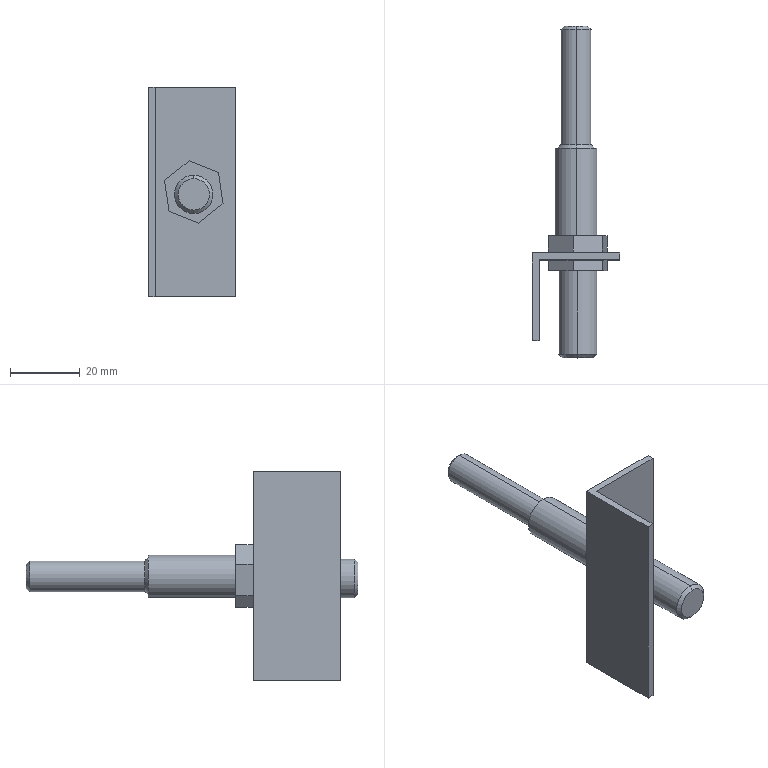Part | SolidWorks | features ICE 4, Chamfer 1, ExtruThin 1 | 1 solid | 37 faces | box 25 x 95 x 60 mm | volume 14738 mm3 | plane 25 | cone 6 | cylinder 6 | commonest cylinder face diameters 8.745 x2 11 x2 12 x2
STEP:
#1=CARTESIAN_POINT('',(12.519,90.,33.288));
#2=VERTEX_POINT('',#1);
#3=CARTESIAN_POINT('',(12.519,90.,26.543));
#4=VERTEX_POINT('',#3);
#5=CARTESIAN_POINT('',(12.519,90.,29.915));
#6=DIRECTION('',(0.,1.,0.));
#7=DIRECTION('',(0.,0.,1.));
#8=AXIS2_PLACEMENT_3D('',#5,#6,#7);
#9=CIRCLE('',#8,3.373);
#10=EDGE_CURVE('',#2,#4,#9,.T.);
#11=ORIENTED_EDGE('',*,*,#10,.F.);
#12=CARTESIAN_POINT('',(12.519,89.,34.288));
#13=VERTEX_POINT('',#12);
#14=CARTESIAN_POINT('',(12.519,90.,33.288));
#15=DIRECTION('',(0.,-0.7071,0.7071));
#16=VECTOR('',#15,1000.);
#17=LINE('',#14,#16);
#18=EDGE_CURVE('',#2,#13,#17,.T.);
#19=ORIENTED_EDGE('',*,*,#18,.T.);
#20=CARTESIAN_POINT('',(12.519,89.,25.543));
#21=VERTEX_POINT('',#20);
#22=CARTESIAN_POINT('',(12.519,89.,29.915));
#23=DIRECTION('',(0.,-1.,0.));
#24=DIRECTION('',(0.,0.,1.));
#25=AXIS2_PLACEMENT_3D('',#22,#23,#24);
#26=CIRCLE('',#25,4.373);
#27=EDGE_CURVE('',#21,#13,#26,.T.);
#28=ORIENTED_EDGE('',*,*,#27,.F.);
#29=CARTESIAN_POINT('',(12.519,90.,26.543));
#30=DIRECTION('',(0.,-0.7071,-0.7071));
#31=VECTOR('',#30,1000.);
#32=LINE('',#29,#31);
#33=EDGE_CURVE('',#4,#21,#32,.T.);
#34=ORIENTED_EDGE('',*,*,#33,.F.);
#35=EDGE_LOOP('',(#11,#19,#28,#34));
#36=FACE_OUTER_BOUND('',#35,.T.);
#37=CARTESIAN_POINT('',(12.519,90.,29.915));
#38=DIRECTION('',(0.,-1.,0.));
#39=DIRECTION('',(0.,0.,-1.));
#40=AXIS2_PLACEMENT_3D('',#37,#38,#39);
#41=CONICAL_SURFACE('',#40,3.373,0.7854);
#42=ADVANCED_FACE('',(#36),#41,.T.);
#43=CARTESIAN_POINT('',(13.,-5.,24.819));
#44=VERTEX_POINT('',#43);
#45=CARTESIAN_POINT('',(13.,-5.,33.819));
#46=VERTEX_POINT('',#45);
#47=CARTESIAN_POINT('',(13.,-5.,29.319));
#48=DIRECTION('',(0.,-1.,0.));
#49=DIRECTION('',(0.,0.,-1.));
#50=AXIS2_PLACEMENT_3D('',#47,#48,#49);
#51=CIRCLE('',#50,4.5);
#52=EDGE_CURVE('',#44,#46,#51,.T.);
#53=ORIENTED_EDGE('',*,*,#52,.F.);
#54=CARTESIAN_POINT('',(13.,-4.,23.819));
#55=VERTEX_POINT('',#54);
#56=CARTESIAN_POINT('',(13.,-5.,24.819));
#57=DIRECTION('',(0.,0.7071,-0.7071));
#58=VECTOR('',#57,1000.);
#59=LINE('',#56,#58);
#60=EDGE_CURVE('',#44,#55,#59,.T.);
#61=ORIENTED_EDGE('',*,*,#60,.T.);
#62=CARTESIAN_POINT('',(13.,-4.,34.819));
#63=VERTEX_POINT('',#62);
#64=CARTESIAN_POINT('',(13.,-4.,29.319));
#65=DIRECTION('',(0.,1.,0.));
#66=DIRECTION('',(0.,0.,-1.));
#67=AXIS2_PLACEMENT_3D('',#64,#65,#66);
#68=CIRCLE('',#67,5.5);
#69=EDGE_CURVE('',#63,#55,#68,.T.);
#70=ORIENTED_EDGE('',*,*,#69,.F.);
#71=CARTESIAN_POINT('',(13.,-5.,33.819));
#72=DIRECTION('',(0.,0.7071,0.7071));
#73=VECTOR('',#72,1000.);
#74=LINE('',#71,#73);
#75=EDGE_CURVE('',#46,#63,#74,.T.);
#76=ORIENTED_EDGE('',*,*,#75,.F.);
#77=EDGE_LOOP('',(#53,#61,#70,#76));
#78=FACE_OUTER_BOUND('',#77,.T.);
#79=CARTESIAN_POINT('',(13.,-5.,29.319));
#80=DIRECTION('',(0.,1.,0.));
#81=DIRECTION('',(0.,0.,1.));
#82=AXIS2_PLACEMENT_3D('',#79,#80,#81);
#83=CONICAL_SURFACE('',#82,4.5,0.7854);
#84=ADVANCED_FACE('',(#78),#83,.T.);
#85=CARTESIAN_POINT('',(12.519,56.,34.288));
#86=VERTEX_POINT('',#85);
#87=CARTESIAN_POINT('',(12.519,56.,25.543));
#88=VERTEX_POINT('',#87);
#89=CARTESIAN_POINT('',(12.519,56.,29.915));
#90=DIRECTION('',(0.,1.,0.));
#91=DIRECTION('',(0.,0.,1.));
#92=AXIS2_PLACEMENT_3D('',#89,#90,#91);
#93=CIRCLE('',#92,4.373);
#94=EDGE_CURVE('',#86,#88,#93,.T.);
#95=ORIENTED_EDGE('',*,*,#94,.F.);
#96=CARTESIAN_POINT('',(12.519,55.,35.288));
#97=VERTEX_POINT('',#96);
#98=CARTESIAN_POINT('',(12.519,56.,34.288));
#99=DIRECTION('',(0.,-0.7071,0.7071));
#100=VECTOR('',#99,1000.);
#101=LINE('',#98,#100);
#102=EDGE_CURVE('',#86,#97,#101,.T.);
#103=ORIENTED_EDGE('',*,*,#102,.T.);
#104=CARTESIAN_POINT('',(12.519,55.,24.543));
#105=VERTEX_POINT('',#104);
#106=CARTESIAN_POINT('',(12.519,55.,29.915));
#107=DIRECTION('',(0.,-1.,0.));
#108=DIRECTION('',(0.,0.,1.));
#109=AXIS2_PLACEMENT_3D('',#106,#107,#108);
#110=CIRCLE('',#109,5.373);
#111=EDGE_CURVE('',#105,#97,#110,.T.);
#112=ORIENTED_EDGE('',*,*,#111,.F.);
#113=CARTESIAN_POINT('',(12.519,56.,25.543));
#114=DIRECTION('',(0.,-0.7071,-0.7071));
#115=VECTOR('',#114,1000.);
#116=LINE('',#113,#115);
#117=EDGE_CURVE('',#88,#105,#116,.T.);
#118=ORIENTED_EDGE('',*,*,#117,.F.);
#119=EDGE_LOOP('',(#95,#103,#112,#118));
#120=FACE_OUTER_BOUND('',#119,.T.);
#121=CARTESIAN_POINT('',(12.519,56.,29.915));
#122=DIRECTION('',(0.,-1.,0.));
#123=DIRECTION('',(0.,0.,-1.));
#124=AXIS2_PLACEMENT_3D('',#121,#122,#123);
#125=CONICAL_SURFACE('',#124,4.373,0.7854);
#126=ADVANCED_FACE('',(#120),#125,.T.);
#127=ORIENTED_EDGE('',*,*,#27,.T.);
#128=CARTESIAN_POINT('',(12.519,90.,34.288));
#129=DIRECTION('',(0.,-1.,0.));
#130=VECTOR('',#129,1000.);
#131=LINE('',#128,#130);
#132=EDGE_CURVE('',#13,#86,#131,.T.);
#133=ORIENTED_EDGE('',*,*,#132,.T.);
#134=ORIENTED_EDGE('',*,*,#94,.T.);
#135=CARTESIAN_POINT('',(12.519,90.,25.543));
#136=DIRECTION('',(0.,-1.,0.));
#137=VECTOR('',#136,1000.);
#138=LINE('',#135,#137);
#139=EDGE_CURVE('',#21,#88,#138,.T.);
#140=ORIENTED_EDGE('',*,*,#139,.F.);
#141=EDGE_LOOP('',(#127,#133,#134,#140));
#142=FACE_OUTER_BOUND('',#141,.T.);
#143=CARTESIAN_POINT('',(12.519,90.,29.915));
#144=DIRECTION('',(0.,-1.,0.));
#145=DIRECTION('',(0.,0.,-1.));
#146=AXIS2_PLACEMENT_3D('',#143,#144,#145);
#147=CYLINDRICAL_SURFACE('',#146,4.373);
#148=ADVANCED_FACE('',(#142),#147,.T.);
#149=CARTESIAN_POINT('',(12.519,55.,35.915));
#150=VERTEX_POINT('',#149);
#151=CARTESIAN_POINT('',(12.519,55.,23.915));
#152=VERTEX_POINT('',#151);
#153=CARTESIAN_POINT('',(12.519,55.,29.915));
#154=DIRECTION('',(0.,1.,0.));
#155=DIRECTION('',(0.,0.,1.));
#156=AXIS2_PLACEMENT_3D('',#153,#154,#155);
#157=CIRCLE('',#156,6.);
#158=EDGE_CURVE('',#150,#152,#157,.T.);
#159=ORIENTED_EDGE('',*,*,#158,.F.);
#160=CARTESIAN_POINT('',(12.519,30.,35.915));
#161=VERTEX_POINT('',#160);
#162=CARTESIAN_POINT('',(12.519,55.,35.915));
#163=DIRECTION('',(0.,-1.,0.));
#164=VECTOR('',#163,1000.);
#165=LINE('',#162,#164);
#166=EDGE_CURVE('',#150,#161,#165,.T.);
#167=ORIENTED_EDGE('',*,*,#166,.T.);
#168=CARTESIAN_POINT('',(12.519,30.,23.915));
#169=VERTEX_POINT('',#168);
#170=CARTESIAN_POINT('',(12.519,30.,29.915));
#171=DIRECTION('',(0.,1.,0.));
#172=DIRECTION('',(0.,0.,1.));
#173=AXIS2_PLACEMENT_3D('',#170,#171,#172);
#174=CIRCLE('',#173,6.);
#175=EDGE_CURVE('',#161,#169,#174,.T.);
#176=ORIENTED_EDGE('',*,*,#175,.T.);
#177=CARTESIAN_POINT('',(12.519,55.,23.915));
#178=DIRECTION('',(0.,-1.,0.));
#179=VECTOR('',#178,1000.);
#180=LINE('',#177,#179);
#181=EDGE_CURVE('',#152,#169,#180,.T.);
#182=ORIENTED_EDGE('',*,*,#181,.F.);
#183=EDGE_LOOP('',(#159,#167,#176,#182));
#184=FACE_OUTER_BOUND('',#183,.T.);
#185=CARTESIAN_POINT('',(12.519,55.,29.915));
#186=DIRECTION('',(0.,-1.,0.));
#187=DIRECTION('',(0.,0.,-1.));
#188=AXIS2_PLACEMENT_3D('',#185,#186,#187);
#189=CYLINDRICAL_SURFACE('',#188,6.);
#190=ADVANCED_FACE('',(#184),#189,.T.);
#191=ORIENTED_EDGE('',*,*,#69,.T.);
#192=CARTESIAN_POINT('',(13.,20.,23.819));
#193=VERTEX_POINT('',#192);
#194=CARTESIAN_POINT('',(13.,-5.,23.819));
#195=DIRECTION('',(0.,1.,0.));
#196=VECTOR('',#195,1000.);
#197=LINE('',#194,#196);
#198=EDGE_CURVE('',#55,#193,#197,.T.);
#199=ORIENTED_EDGE('',*,*,#198,.T.);
#200=CARTESIAN_POINT('',(13.,20.,34.819));
#201=VERTEX_POINT('',#200);
#202=CARTESIAN_POINT('',(13.,20.,29.319));
#203=DIRECTION('',(0.,-1.,0.));
#204=DIRECTION('',(0.,0.,1.));
#205=AXIS2_PLACEMENT_3D('',#202,#203,#204);
#206=CIRCLE('',#205,5.5);
#207=EDGE_CURVE('',#193,#201,#206,.T.);
#208=ORIENTED_EDGE('',*,*,#207,.T.);
#209=CARTESIAN_POINT('',(13.,-5.,34.819));
#210=DIRECTION('',(0.,1.,0.));
#211=VECTOR('',#210,1000.);
#212=LINE('',#209,#211);
#213=EDGE_CURVE('',#63,#201,#212,.T.);
#214=ORIENTED_EDGE('',*,*,#213,.F.);
#215=EDGE_LOOP('',(#191,#199,#208,#214));
#216=FACE_OUTER_BOUND('',#215,.T.);
#217=CARTESIAN_POINT('',(13.,-5.,29.319));
#218=DIRECTION('',(0.,1.,0.));
#219=DIRECTION('',(0.,0.,1.));
#220=AXIS2_PLACEMENT_3D('',#217,#218,#219);
#221=CYLINDRICAL_SURFACE('',#220,5.5);
#222=ADVANCED_FACE('',(#216),#221,.T.);
#223=CARTESIAN_POINT('',(2.,23.,0.));
#224=VERTEX_POINT('',#223);
#225=CARTESIAN_POINT('',(25.,23.,0.));
#226=VERTEX_POINT('',#225);
#227=CARTESIAN_POINT('',(0.,23.,0.));
#228=DIRECTION('',(1.,0.,0.));
#229=VECTOR('',#228,1000.);
#230=LINE('',#227,#229);
#231=EDGE_CURVE('',#224,#226,#230,.T.);
#232=ORIENTED_EDGE('',*,*,#231,.T.);
#233=CARTESIAN_POINT('',(25.,23.,60.));
#234=VERTEX_POINT('',#233);
#235=CARTESIAN_POINT('',(25.,23.,60.));
#236=DIRECTION('',(0.,0.,-1.));
#237=VECTOR('',#236,1000.);
#238=LINE('',#235,#237);
#239=EDGE_CURVE('',#234,#226,#238,.T.);
#240=ORIENTED_EDGE('',*,*,#239,.F.);
#241=CARTESIAN_POINT('',(2.,23.,60.));
#242=VERTEX_POINT('',#241);
#243=CARTESIAN_POINT('',(0.,23.,60.));
#244=DIRECTION('',(1.,0.,0.));
#245=VECTOR('',#244,1000.);
#246=LINE('',#243,#245);
#247=EDGE_CURVE('',#242,#234,#246,.T.);
#248=ORIENTED_EDGE('',*,*,#247,.F.);
#249=CARTESIAN_POINT('',(2.,23.,60.));
#250=DIRECTION('',(0.,0.,-1.));
#251=VECTOR('',#250,1000.);
#252=LINE('',#249,#251);
#253=EDGE_CURVE('',#242,#224,#252,.T.);
#254=ORIENTED_EDGE('',*,*,#253,.T.);
#255=EDGE_LOOP('',(#232,#240,#248,#254));
#256=FACE_OUTER_BOUND('',#255,.T.);
#257=CARTESIAN_POINT('',(11.685,23.,38.911));
#258=VERTEX_POINT('',#257);
#259=CARTESIAN_POINT('',(4.625,23.,33.317));
#260=VERTEX_POINT('',#259);
#261=CARTESIAN_POINT('',(14.773,23.,41.358));
#262=DIRECTION('',(-0.7837,0.,-0.6211));
#263=VECTOR('',#262,1000.);
#264=LINE('',#261,#263);
#265=EDGE_CURVE('',#258,#260,#264,.T.);
#266=ORIENTED_EDGE('',*,*,#265,.F.);
#267=CARTESIAN_POINT('',(20.06,23.,35.594));
#268=VERTEX_POINT('',#267);
#269=CARTESIAN_POINT('',(-5.635,23.,45.77));
#270=DIRECTION('',(-0.9297,0.,0.3682));
#271=VECTOR('',#270,1000.);
#272=LINE('',#269,#271);
#273=EDGE_CURVE('',#268,#258,#272,.T.);
#274=ORIENTED_EDGE('',*,*,#273,.F.);
#275=CARTESIAN_POINT('',(21.375,23.,26.683));
#276=VERTEX_POINT('',#275);
#277=CARTESIAN_POINT('',(16.107,23.,62.377));
#278=DIRECTION('',(-0.146,0.,0.9893));
#279=VECTOR('',#278,1000.);
#280=LINE('',#277,#279);
#281=EDGE_CURVE('',#276,#268,#280,.T.);
#282=ORIENTED_EDGE('',*,*,#281,.F.);
#283=CARTESIAN_POINT('',(14.315,23.,21.089));
#284=VERTEX_POINT('',#283);
#285=CARTESIAN_POINT('',(24.463,23.,29.13));
#286=DIRECTION('',(0.7837,0.,0.6211));
#287=VECTOR('',#286,1000.);
#288=LINE('',#285,#287);
#289=EDGE_CURVE('',#284,#276,#288,.T.);
#290=ORIENTED_EDGE('',*,*,#289,.F.);
#291=CARTESIAN_POINT('',(5.94,23.,24.406));
#292=VERTEX_POINT('',#291);
#293=CARTESIAN_POINT('',(-11.38,23.,31.265));
#294=DIRECTION('',(0.9297,0.,-0.3682));
#295=VECTOR('',#294,1000.);
#296=LINE('',#293,#295);
#297=EDGE_CURVE('',#292,#284,#296,.T.);
#298=ORIENTED_EDGE('',*,*,#297,.F.);
#299=CARTESIAN_POINT('',(0.6727,23.,60.099));
#300=DIRECTION('',(0.146,0.,-0.9893));
#301=VECTOR('',#300,1000.);
#302=LINE('',#299,#301);
#303=EDGE_CURVE('',#260,#292,#302,.T.);
#304=ORIENTED_EDGE('',*,*,#303,.F.);
#305=EDGE_LOOP('',(#266,#274,#282,#290,#298,#304));
#306=FACE_BOUND('',#305,.T.);
#307=CARTESIAN_POINT('',(0.,23.,60.));
#308=DIRECTION('',(0.,1.,0.));
#309=DIRECTION('',(0.,0.,1.));
#310=AXIS2_PLACEMENT_3D('',#307,#308,#309);
#311=PLANE('',#310);
#312=ADVANCED_FACE('',(#256,#306),#311,.F.);
#313=CARTESIAN_POINT('',(0.,25.,0.));
#314=VERTEX_POINT('',#313);
#315=CARTESIAN_POINT('',(25.,25.,0.));
#316=VERTEX_POINT('',#315);
#317=CARTESIAN_POINT('',(0.,25.,0.));
#318=DIRECTION('',(1.,0.,0.));
#319=VECTOR('',#318,1000.);
#320=LINE('',#317,#319);
#321=EDGE_CURVE('',#314,#316,#320,.T.);
#322=ORIENTED_EDGE('',*,*,#321,.F.);
#323=CARTESIAN_POINT('',(0.,25.,60.));
#324=VERTEX_POINT('',#323);
#325=CARTESIAN_POINT('',(0.,25.,60.));
#326=DIRECTION('',(0.,0.,-1.));
#327=VECTOR('',#326,1000.);
#328=LINE('',#325,#327);
#329=EDGE_CURVE('',#324,#314,#328,.T.);
#330=ORIENTED_EDGE('',*,*,#329,.F.);
#331=CARTESIAN_POINT('',(25.,25.,60.));
#332=VERTEX_POINT('',#331);
#333=CARTESIAN_POINT('',(0.,25.,60.));
#334=DIRECTION('',(1.,0.,0.));
#335=VECTOR('',#334,1000.);
#336=LINE('',#333,#335);
#337=EDGE_CURVE('',#324,#332,#336,.T.);
#338=ORIENTED_EDGE('',*,*,#337,.T.);
#339=CARTESIAN_POINT('',(25.,25.,60.));
#340=DIRECTION('',(0.,0.,-1.));
#341=VECTOR('',#340,1000.);
#342=LINE('',#339,#341);
#343=EDGE_CURVE('',#332,#316,#342,.T.);
#344=ORIENTED_EDGE('',*,*,#343,.T.);
#345=EDGE_LOOP('',(#322,#330,#338,#344));
#346=FACE_OUTER_BOUND('',#345,.T.);
#347=CARTESIAN_POINT('',(20.06,25.,35.594));
#348=VERTEX_POINT('',#347);
#349=CARTESIAN_POINT('',(11.685,25.,38.911));
#350=VERTEX_POINT('',#349);
#351=CARTESIAN_POINT('',(-5.635,25.,45.77));
#352=DIRECTION('',(-0.9297,0.,0.3682));
#353=VECTOR('',#352,1000.);
#354=LINE('',#351,#353);
#355=EDGE_CURVE('',#348,#350,#354,.T.);
#356=ORIENTED_EDGE('',*,*,#355,.T.);
#357=CARTESIAN_POINT('',(4.625,25.,33.317));
#358=VERTEX_POINT('',#357);
#359=CARTESIAN_POINT('',(14.773,25.,41.358));
#360=DIRECTION('',(-0.7837,0.,-0.6211));
#361=VECTOR('',#360,1000.);
#362=LINE('',#359,#361);
#363=EDGE_CURVE('',#350,#358,#362,.T.);
#364=ORIENTED_EDGE('',*,*,#363,.T.);
#365=CARTESIAN_POINT('',(5.94,25.,24.406));
#366=VERTEX_POINT('',#365);
#367=CARTESIAN_POINT('',(0.6727,25.,60.099));
#368=DIRECTION('',(0.146,0.,-0.9893));
#369=VECTOR('',#368,1000.);
#370=LINE('',#367,#369);
#371=EDGE_CURVE('',#358,#366,#370,.T.);
#372=ORIENTED_EDGE('',*,*,#371,.T.);
#373=CARTESIAN_POINT('',(14.315,25.,21.089));
#374=VERTEX_POINT('',#373);
#375=CARTESIAN_POINT('',(-11.38,25.,31.265));
#376=DIRECTION('',(0.9297,0.,-0.3682));
#377=VECTOR('',#376,1000.);
#378=LINE('',#375,#377);
#379=EDGE_CURVE('',#366,#374,#378,.T.);
#380=ORIENTED_EDGE('',*,*,#379,.T.);
#381=CARTESIAN_POINT('',(21.375,25.,26.683));
#382=VERTEX_POINT('',#381);
#383=CARTESIAN_POINT('',(24.463,25.,29.13));
#384=DIRECTION('',(0.7837,0.,0.6211));
#385=VECTOR('',#384,1000.);
#386=LINE('',#383,#385);
#387=EDGE_CURVE('',#374,#382,#386,.T.);
#388=ORIENTED_EDGE('',*,*,#387,.T.);
#389=CARTESIAN_POINT('',(16.107,25.,62.377));
#390=DIRECTION('',(-0.146,0.,0.9893));
#391=VECTOR('',#390,1000.);
#392=LINE('',#389,#391);
#393=EDGE_CURVE('',#382,#348,#392,.T.);
#394=ORIENTED_EDGE('',*,*,#393,.T.);
#395=EDGE_LOOP('',(#356,#364,#372,#380,#388,#394));
#396=FACE_BOUND('',#395,.T.);
#397=CARTESIAN_POINT('',(0.,25.,60.));
#398=DIRECTION('',(0.,1.,0.));
#399=DIRECTION('',(0.,0.,1.));
#400=AXIS2_PLACEMENT_3D('',#397,#398,#399);
#401=PLANE('',#400);
#402=ADVANCED_FACE('',(#346,#396),#401,.T.);
#403=CARTESIAN_POINT('',(25.,25.,0.));
#404=DIRECTION('',(0.,-1.,0.));
#405=VECTOR('',#404,1000.);
#406=LINE('',#403,#405);
#407=EDGE_CURVE('',#316,#226,#406,.T.);
#408=ORIENTED_EDGE('',*,*,#407,.F.);
#409=ORIENTED_EDGE('',*,*,#343,.F.);
#410=CARTESIAN_POINT('',(25.,25.,60.));
#411=DIRECTION('',(0.,-1.,0.));
#412=VECTOR('',#411,1000.);
#413=LINE('',#410,#412);
#414=EDGE_CURVE('',#332,#234,#413,.T.);
#415=ORIENTED_EDGE('',*,*,#414,.T.);
#416=ORIENTED_EDGE('',*,*,#239,.T.);
#417=EDGE_LOOP('',(#408,#409,#415,#416));
#418=FACE_OUTER_BOUND('',#417,.T.);
#419=CARTESIAN_POINT('',(25.,25.,60.));
#420=DIRECTION('',(1.,0.,0.));
#421=DIRECTION('',(0.,0.,-1.));
#422=AXIS2_PLACEMENT_3D('',#419,#420,#421);
#423=PLANE('',#422);
#424=ADVANCED_FACE('',(#418),#423,.T.);
#425=CARTESIAN_POINT('',(0.,0.,0.));
#426=VERTEX_POINT('',#425);
#427=CARTESIAN_POINT('',(0.,0.,0.));
#428=DIRECTION('',(0.,1.,0.));
#429=VECTOR('',#428,1000.);
#430=LINE('',#427,#429);
#431=EDGE_CURVE('',#426,#314,#430,.T.);
#432=ORIENTED_EDGE('',*,*,#431,.F.);
#433=CARTESIAN_POINT('',(0.,0.,60.));
#434=VERTEX_POINT('',#433);
#435=CARTESIAN_POINT('',(0.,0.,60.));
#436=DIRECTION('',(0.,0.,-1.));
#437=VECTOR('',#436,1000.);
#438=LINE('',#435,#437);
#439=EDGE_CURVE('',#434,#426,#438,.T.);
#440=ORIENTED_EDGE('',*,*,#439,.F.);
#441=CARTESIAN_POINT('',(0.,0.,60.));
#442=DIRECTION('',(0.,1.,0.));
#443=VECTOR('',#442,1000.);
#444=LINE('',#441,#443);
#445=EDGE_CURVE('',#434,#324,#444,.T.);
#446=ORIENTED_EDGE('',*,*,#445,.T.);
#447=ORIENTED_EDGE('',*,*,#329,.T.);
#448=EDGE_LOOP('',(#432,#440,#446,#447));
#449=FACE_OUTER_BOUND('',#448,.T.);
#450=CARTESIAN_POINT('',(0.,0.,60.));
#451=DIRECTION('',(-1.,0.,0.));
#452=DIRECTION('',(0.,0.,1.));
#453=AXIS2_PLACEMENT_3D('',#450,#451,#452);
#454=PLANE('',#453);
#455=ADVANCED_FACE('',(#449),#454,.T.);
#456=CARTESIAN_POINT('',(2.,0.,0.));
#457=VERTEX_POINT('',#456);
#458=CARTESIAN_POINT('',(2.,0.,0.));
#459=DIRECTION('',(-1.,0.,0.));
#460=VECTOR('',#459,1000.);
#461=LINE('',#458,#460);
#462=EDGE_CURVE('',#457,#426,#461,.T.);
#463=ORIENTED_EDGE('',*,*,#462,.F.);
#464=CARTESIAN_POINT('',(2.,0.,60.));
#465=VERTEX_POINT('',#464);
#466=CARTESIAN_POINT('',(2.,0.,60.));
#467=DIRECTION('',(0.,0.,-1.));
#468=VECTOR('',#467,1000.);
#469=LINE('',#466,#468);
#470=EDGE_CURVE('',#465,#457,#469,.T.);
#471=ORIENTED_EDGE('',*,*,#470,.F.);
#472=CARTESIAN_POINT('',(2.,0.,60.));
#473=DIRECTION('',(-1.,0.,0.));
#474=VECTOR('',#473,1000.);
#475=LINE('',#472,#474);
#476=EDGE_CURVE('',#465,#434,#475,.T.);
#477=ORIENTED_EDGE('',*,*,#476,.T.);
#478=ORIENTED_EDGE('',*,*,#439,.T.);
#479=EDGE_LOOP('',(#463,#471,#477,#478));
#480=FACE_OUTER_BOUND('',#479,.T.);
#481=CARTESIAN_POINT('',(2.,0.,60.));
#482=DIRECTION('',(0.,-1.,0.));
#483=DIRECTION('',(0.,0.,-1.));
#484=AXIS2_PLACEMENT_3D('',#481,#482,#483);
#485=PLANE('',#484);
#486=ADVANCED_FACE('',(#480),#485,.T.);
#487=CARTESIAN_POINT('',(2.,0.,0.));
#488=DIRECTION('',(0.,1.,0.));
#489=VECTOR('',#488,1000.);
#490=LINE('',#487,#489);
#491=EDGE_CURVE('',#457,#224,#490,.T.);
#492=ORIENTED_EDGE('',*,*,#491,.T.);
#493=ORIENTED_EDGE('',*,*,#253,.F.);
#494=CARTESIAN_POINT('',(2.,0.,60.));
#495=DIRECTION('',(0.,1.,0.));
#496=VECTOR('',#495,1000.);
#497=LINE('',#494,#496);
#498=EDGE_CURVE('',#465,#242,#497,.T.);
#499=ORIENTED_EDGE('',*,*,#498,.F.);
#500=ORIENTED_EDGE('',*,*,#470,.T.);
#501=EDGE_LOOP('',(#492,#493,#499,#500));
#502=FACE_OUTER_BOUND('',#501,.T.);
#503=CARTESIAN_POINT('',(2.,0.,60.));
#504=DIRECTION('',(-1.,0.,0.));
#505=DIRECTION('',(0.,0.,1.));
#506=AXIS2_PLACEMENT_3D('',#503,#504,#505);
#507=PLANE('',#506);
#508=ADVANCED_FACE('',(#502),#507,.F.);
#509=ORIENTED_EDGE('',*,*,#247,.T.);
#510=ORIENTED_EDGE('',*,*,#414,.F.);
#511=ORIENTED_EDGE('',*,*,#337,.F.);
#512=ORIENTED_EDGE('',*,*,#445,.F.);
#513=ORIENTED_EDGE('',*,*,#476,.F.);
#514=ORIENTED_EDGE('',*,*,#498,.T.);
#515=EDGE_LOOP('',(#509,#510,#511,#512,#513,#514));
#516=FACE_OUTER_BOUND('',#515,.T.);
#517=CARTESIAN_POINT('',(0.,0.,60.));
#518=DIRECTION('',(0.,0.,-1.));
#519=DIRECTION('',(-1.,0.,0.));
#520=AXIS2_PLACEMENT_3D('',#517,#518,#519);
#521=PLANE('',#520);
#522=ADVANCED_FACE('',(#516),#521,.F.);
#523=ORIENTED_EDGE('',*,*,#231,.F.);
#524=ORIENTED_EDGE('',*,*,#491,.F.);
#525=ORIENTED_EDGE('',*,*,#462,.T.);
#526=ORIENTED_EDGE('',*,*,#431,.T.);
#527=ORIENTED_EDGE('',*,*,#321,.T.);
#528=ORIENTED_EDGE('',*,*,#407,.T.);
#529=EDGE_LOOP('',(#523,#524,#525,#526,#527,#528));
#530=FACE_OUTER_BOUND('',#529,.T.);
#531=CARTESIAN_POINT('',(0.,0.,0.));
#532=DIRECTION('',(0.,0.,-1.));
#533=DIRECTION('',(-1.,0.,0.));
#534=AXIS2_PLACEMENT_3D('',#531,#532,#533);
#535=PLANE('',#534);
#536=ADVANCED_FACE('',(#530),#535,.T.);
#537=CARTESIAN_POINT('',(12.519,30.,29.915));
#538=DIRECTION('',(0.,1.,0.));
#539=DIRECTION('',(0.,0.,1.));
#540=AXIS2_PLACEMENT_3D('',#537,#538,#539);
#541=CIRCLE('',#540,6.);
#542=EDGE_CURVE('',#169,#161,#541,.T.);
#543=ORIENTED_EDGE('',*,*,#542,.F.);
#544=ORIENTED_EDGE('',*,*,#175,.F.);
#545=EDGE_LOOP('',(#543,#544));
#546=FACE_BOUND('',#545,.T.);
#547=CARTESIAN_POINT('',(4.625,30.,33.317));
#548=VERTEX_POINT('',#547);
#549=CARTESIAN_POINT('',(11.685,30.,38.911));
#550=VERTEX_POINT('',#549);
#551=CARTESIAN_POINT('',(4.625,30.,33.317));
#552=DIRECTION('',(0.7837,0.,0.6211));
#553=VECTOR('',#552,1000.);
#554=LINE('',#551,#553);
#555=EDGE_CURVE('',#548,#550,#554,.T.);
#556=ORIENTED_EDGE('',*,*,#555,.T.);
#557=CARTESIAN_POINT('',(20.06,30.,35.594));
#558=VERTEX_POINT('',#557);
#559=CARTESIAN_POINT('',(11.685,30.,38.911));
#560=DIRECTION('',(0.9297,0.,-0.3682));
#561=VECTOR('',#560,1000.);
#562=LINE('',#559,#561);
#563=EDGE_CURVE('',#550,#558,#562,.T.);
#564=ORIENTED_EDGE('',*,*,#563,.T.);
#565=CARTESIAN_POINT('',(21.375,30.,26.683));
#566=VERTEX_POINT('',#565);
#567=CARTESIAN_POINT('',(20.06,30.,35.594));
#568=DIRECTION('',(0.146,0.,-0.9893));
#569=VECTOR('',#568,1000.);
#570=LINE('',#567,#569);
#571=EDGE_CURVE('',#558,#566,#570,.T.);
#572=ORIENTED_EDGE('',*,*,#571,.T.);
#573=CARTESIAN_POINT('',(14.315,30.,21.089));
#574=VERTEX_POINT('',#573);
#575=CARTESIAN_POINT('',(21.375,30.,26.683));
#576=DIRECTION('',(-0.7837,0.,-0.6211));
#577=VECTOR('',#576,1000.);
#578=LINE('',#575,#577);
#579=EDGE_CURVE('',#566,#574,#578,.T.);
#580=ORIENTED_EDGE('',*,*,#579,.T.);
#581=CARTESIAN_POINT('',(5.94,30.,24.406));
#582=VERTEX_POINT('',#581);
#583=CARTESIAN_POINT('',(14.315,30.,21.089));
#584=DIRECTION('',(-0.9297,0.,0.3682));
#585=VECTOR('',#584,1000.);
#586=LINE('',#583,#585);
#587=EDGE_CURVE('',#574,#582,#586,.T.);
#588=ORIENTED_EDGE('',*,*,#587,.T.);
#589=CARTESIAN_POINT('',(5.94,30.,24.406));
#590=DIRECTION('',(-0.146,0.,0.9893));
#591=VECTOR('',#590,1000.);
#592=LINE('',#589,#591);
#593=EDGE_CURVE('',#582,#548,#592,.T.);
#594=ORIENTED_EDGE('',*,*,#593,.T.);
#595=EDGE_LOOP('',(#556,#564,#572,#580,#588,#594));
#596=FACE_OUTER_BOUND('',#595,.T.);
#597=CARTESIAN_POINT('',(0.,30.,0.));
#598=DIRECTION('',(0.,1.,0.));
#599=DIRECTION('',(0.,0.,1.));
#600=AXIS2_PLACEMENT_3D('',#597,#598,#599);
#601=PLANE('',#600);
#602=ADVANCED_FACE('',(#546,#596),#601,.T.);
#603=ORIENTED_EDGE('',*,*,#371,.F.);
#604=CARTESIAN_POINT('',(4.625,30.,33.317));
#605=DIRECTION('',(0.,-1.,0.));
#606=VECTOR('',#605,1000.);
#607=LINE('',#604,#606);
#608=EDGE_CURVE('',#548,#358,#607,.T.);
#609=ORIENTED_EDGE('',*,*,#608,.F.);
#610=ORIENTED_EDGE('',*,*,#593,.F.);
#611=CARTESIAN_POINT('',(5.94,30.,24.406));
#612=DIRECTION('',(0.,-1.,0.));
#613=VECTOR('',#612,1000.);
#614=LINE('',#611,#613);
#615=EDGE_CURVE('',#582,#366,#614,.T.);
#616=ORIENTED_EDGE('',*,*,#615,.T.);
#617=EDGE_LOOP('',(#603,#609,#610,#616));
#618=FACE_OUTER_BOUND('',#617,.T.);
#619=CARTESIAN_POINT('',(5.94,30.,24.406));
#620=DIRECTION('',(0.9893,0.,0.146));
#621=DIRECTION('',(0.146,0.,-0.9893));
#622=AXIS2_PLACEMENT_3D('',#619,#620,#621);
#623=PLANE('',#622);
#624=ADVANCED_FACE('',(#618),#623,.F.);
#625=ORIENTED_EDGE('',*,*,#379,.F.);
#626=ORIENTED_EDGE('',*,*,#615,.F.);
#627=ORIENTED_EDGE('',*,*,#587,.F.);
#628=CARTESIAN_POINT('',(14.315,30.,21.089));
#629=DIRECTION('',(0.,-1.,0.));
#630=VECTOR('',#629,1000.);
#631=LINE('',#628,#630);
#632=EDGE_CURVE('',#574,#374,#631,.T.);
#633=ORIENTED_EDGE('',*,*,#632,.T.);
#634=EDGE_LOOP('',(#625,#626,#627,#633));
#635=FACE_OUTER_BOUND('',#634,.T.);
#636=CARTESIAN_POINT('',(14.315,30.,21.089));
#637=DIRECTION('',(0.3682,0.,0.9297));
#638=DIRECTION('',(0.9297,0.,-0.3682));
#639=AXIS2_PLACEMENT_3D('',#636,#637,#638);
#640=PLANE('',#639);
#641=ADVANCED_FACE('',(#635),#640,.F.);
#642=ORIENTED_EDGE('',*,*,#387,.F.);
#643=ORIENTED_EDGE('',*,*,#632,.F.);
#644=ORIENTED_EDGE('',*,*,#579,.F.);
#645=CARTESIAN_POINT('',(21.375,30.,26.683));
#646=DIRECTION('',(0.,-1.,0.));
#647=VECTOR('',#646,1000.);
#648=LINE('',#645,#647);
#649=EDGE_CURVE('',#566,#382,#648,.T.);
#650=ORIENTED_EDGE('',*,*,#649,.T.);
#651=EDGE_LOOP('',(#642,#643,#644,#650));
#652=FACE_OUTER_BOUND('',#651,.T.);
#653=CARTESIAN_POINT('',(21.375,30.,26.683));
#654=DIRECTION('',(-0.6211,0.,0.7837));
#655=DIRECTION('',(0.7837,0.,0.6211));
#656=AXIS2_PLACEMENT_3D('',#653,#654,#655);
#657=PLANE('',#656);
#658=ADVANCED_FACE('',(#652),#657,.F.);
#659=ORIENTED_EDGE('',*,*,#393,.F.);
#660=ORIENTED_EDGE('',*,*,#649,.F.);
#661=ORIENTED_EDGE('',*,*,#571,.F.);
#662=CARTESIAN_POINT('',(20.06,30.,35.594));
#663=DIRECTION('',(0.,-1.,0.));
#664=VECTOR('',#663,1000.);
#665=LINE('',#662,#664);
#666=EDGE_CURVE('',#558,#348,#665,.T.);
#667=ORIENTED_EDGE('',*,*,#666,.T.);
#668=EDGE_LOOP('',(#659,#660,#661,#667));
#669=FACE_OUTER_BOUND('',#668,.T.);
#670=CARTESIAN_POINT('',(20.06,30.,35.594));
#671=DIRECTION('',(-0.9893,0.,-0.146));
#672=DIRECTION('',(-0.146,0.,0.9893));
#673=AXIS2_PLACEMENT_3D('',#670,#671,#672);
#674=PLANE('',#673);
#675=ADVANCED_FACE('',(#669),#674,.F.);
#676=ORIENTED_EDGE('',*,*,#355,.F.);
#677=ORIENTED_EDGE('',*,*,#666,.F.);
#678=ORIENTED_EDGE('',*,*,#563,.F.);
#679=CARTESIAN_POINT('',(11.685,30.,38.911));
#680=DIRECTION('',(0.,-1.,0.));
#681=VECTOR('',#680,1000.);
#682=LINE('',#679,#681);
#683=EDGE_CURVE('',#550,#350,#682,.T.);
#684=ORIENTED_EDGE('',*,*,#683,.T.);
#685=EDGE_LOOP('',(#676,#677,#678,#684));
#686=FACE_OUTER_BOUND('',#685,.T.);
#687=CARTESIAN_POINT('',(11.685,30.,38.911));
#688=DIRECTION('',(-0.3682,0.,-0.9297));
#689=DIRECTION('',(-0.9297,0.,0.3682));
#690=AXIS2_PLACEMENT_3D('',#687,#688,#689);
#691=PLANE('',#690);
#692=ADVANCED_FACE('',(#686),#691,.F.);
#693=ORIENTED_EDGE('',*,*,#363,.F.);
#694=ORIENTED_EDGE('',*,*,#683,.F.);
#695=ORIENTED_EDGE('',*,*,#555,.F.);
#696=ORIENTED_EDGE('',*,*,#608,.T.);
#697=EDGE_LOOP('',(#693,#694,#695,#696));
#698=FACE_OUTER_BOUND('',#697,.T.);
#699=CARTESIAN_POINT('',(4.625,30.,33.317));
#700=DIRECTION('',(0.6211,0.,-0.7837));
#701=DIRECTION('',(-0.7837,0.,-0.6211));
#702=AXIS2_PLACEMENT_3D('',#699,#700,#701);
#703=PLANE('',#702);
#704=ADVANCED_FACE('',(#698),#703,.F.);
#705=CARTESIAN_POINT('',(11.685,20.,38.911));
#706=VERTEX_POINT('',#705);
#707=CARTESIAN_POINT('',(11.685,30.,38.911));
#708=DIRECTION('',(0.,-1.,0.));
#709=VECTOR('',#708,1000.);
#710=LINE('',#707,#709);
#711=EDGE_CURVE('',#258,#706,#710,.T.);
#712=ORIENTED_EDGE('',*,*,#711,.F.);
#713=ORIENTED_EDGE('',*,*,#265,.T.);
#714=CARTESIAN_POINT('',(4.625,20.,33.317));
#715=VERTEX_POINT('',#714);
#716=CARTESIAN_POINT('',(4.625,30.,33.317));
#717=DIRECTION('',(0.,-1.,0.));
#718=VECTOR('',#717,1000.);
#719=LINE('',#716,#718);
#720=EDGE_CURVE('',#260,#715,#719,.T.);
#721=ORIENTED_EDGE('',*,*,#720,.T.);
#722=CARTESIAN_POINT('',(4.625,20.,33.317));
#723=DIRECTION('',(0.7837,0.,0.6211));
#724=VECTOR('',#723,1000.);
#725=LINE('',#722,#724);
#726=EDGE_CURVE('',#715,#706,#725,.T.);
#727=ORIENTED_EDGE('',*,*,#726,.T.);
#728=EDGE_LOOP('',(#712,#713,#721,#727));
#729=FACE_OUTER_BOUND('',#728,.T.);
#730=CARTESIAN_POINT('',(4.625,30.,33.317));
#731=DIRECTION('',(0.6211,0.,-0.7837));
#732=DIRECTION('',(-0.7837,0.,-0.6211));
#733=AXIS2_PLACEMENT_3D('',#730,#731,#732);
#734=PLANE('',#733);
#735=ADVANCED_FACE('',(#729),#734,.F.);
#736=CARTESIAN_POINT('',(20.06,20.,35.594));
#737=VERTEX_POINT('',#736);
#738=CARTESIAN_POINT('',(20.06,30.,35.594));
#739=DIRECTION('',(0.,-1.,0.));
#740=VECTOR('',#739,1000.);
#741=LINE('',#738,#740);
#742=EDGE_CURVE('',#268,#737,#741,.T.);
#743=ORIENTED_EDGE('',*,*,#742,.F.);
#744=ORIENTED_EDGE('',*,*,#273,.T.);
#745=ORIENTED_EDGE('',*,*,#711,.T.);
#746=CARTESIAN_POINT('',(11.685,20.,38.911));
#747=DIRECTION('',(0.9297,0.,-0.3682));
#748=VECTOR('',#747,1000.);
#749=LINE('',#746,#748);
#750=EDGE_CURVE('',#706,#737,#749,.T.);
#751=ORIENTED_EDGE('',*,*,#750,.T.);
#752=EDGE_LOOP('',(#743,#744,#745,#751));
#753=FACE_OUTER_BOUND('',#752,.T.);
#754=CARTESIAN_POINT('',(11.685,30.,38.911));
#755=DIRECTION('',(-0.3682,0.,-0.9297));
#756=DIRECTION('',(-0.9297,0.,0.3682));
#757=AXIS2_PLACEMENT_3D('',#754,#755,#756);
#758=PLANE('',#757);
#759=ADVANCED_FACE('',(#753),#758,.F.);
#760=CARTESIAN_POINT('',(21.375,20.,26.683));
#761=VERTEX_POINT('',#760);
#762=CARTESIAN_POINT('',(21.375,30.,26.683));
#763=DIRECTION('',(0.,-1.,0.));
#764=VECTOR('',#763,1000.);
#765=LINE('',#762,#764);
#766=EDGE_CURVE('',#276,#761,#765,.T.);
#767=ORIENTED_EDGE('',*,*,#766,.F.);
#768=ORIENTED_EDGE('',*,*,#281,.T.);
#769=ORIENTED_EDGE('',*,*,#742,.T.);
#770=CARTESIAN_POINT('',(20.06,20.,35.594));
#771=DIRECTION('',(0.146,0.,-0.9893));
#772=VECTOR('',#771,1000.);
#773=LINE('',#770,#772);
#774=EDGE_CURVE('',#737,#761,#773,.T.);
#775=ORIENTED_EDGE('',*,*,#774,.T.);
#776=EDGE_LOOP('',(#767,#768,#769,#775));
#777=FACE_OUTER_BOUND('',#776,.T.);
#778=CARTESIAN_POINT('',(20.06,30.,35.594));
#779=DIRECTION('',(-0.9893,0.,-0.146));
#780=DIRECTION('',(-0.146,0.,0.9893));
#781=AXIS2_PLACEMENT_3D('',#778,#779,#780);
#782=PLANE('',#781);
#783=ADVANCED_FACE('',(#777),#782,.F.);
#784=CARTESIAN_POINT('',(14.315,20.,21.089));
#785=VERTEX_POINT('',#784);
#786=CARTESIAN_POINT('',(14.315,30.,21.089));
#787=DIRECTION('',(0.,-1.,0.));
#788=VECTOR('',#787,1000.);
#789=LINE('',#786,#788);
#790=EDGE_CURVE('',#284,#785,#789,.T.);
#791=ORIENTED_EDGE('',*,*,#790,.F.);
#792=ORIENTED_EDGE('',*,*,#289,.T.);
#793=ORIENTED_EDGE('',*,*,#766,.T.);
#794=CARTESIAN_POINT('',(21.375,20.,26.683));
#795=DIRECTION('',(-0.7837,0.,-0.6211));
#796=VECTOR('',#795,1000.);
#797=LINE('',#794,#796);
#798=EDGE_CURVE('',#761,#785,#797,.T.);
#799=ORIENTED_EDGE('',*,*,#798,.T.);
#800=EDGE_LOOP('',(#791,#792,#793,#799));
#801=FACE_OUTER_BOUND('',#800,.T.);
#802=CARTESIAN_POINT('',(21.375,30.,26.683));
#803=DIRECTION('',(-0.6211,0.,0.7837));
#804=DIRECTION('',(0.7837,0.,0.6211));
#805=AXIS2_PLACEMENT_3D('',#802,#803,#804);
#806=PLANE('',#805);
#807=ADVANCED_FACE('',(#801),#806,.F.);
#808=CARTESIAN_POINT('',(5.94,20.,24.406));
#809=VERTEX_POINT('',#808);
#810=CARTESIAN_POINT('',(5.94,30.,24.406));
#811=DIRECTION('',(0.,-1.,0.));
#812=VECTOR('',#811,1000.);
#813=LINE('',#810,#812);
#814=EDGE_CURVE('',#292,#809,#813,.T.);
#815=ORIENTED_EDGE('',*,*,#814,.F.);
#816=ORIENTED_EDGE('',*,*,#297,.T.);
#817=ORIENTED_EDGE('',*,*,#790,.T.);
#818=CARTESIAN_POINT('',(14.315,20.,21.089));
#819=DIRECTION('',(-0.9297,0.,0.3682));
#820=VECTOR('',#819,1000.);
#821=LINE('',#818,#820);
#822=EDGE_CURVE('',#785,#809,#821,.T.);
#823=ORIENTED_EDGE('',*,*,#822,.T.);
#824=EDGE_LOOP('',(#815,#816,#817,#823));
#825=FACE_OUTER_BOUND('',#824,.T.);
#826=CARTESIAN_POINT('',(14.315,30.,21.089));
#827=DIRECTION('',(0.3682,0.,0.9297));
#828=DIRECTION('',(0.9297,0.,-0.3682));
#829=AXIS2_PLACEMENT_3D('',#826,#827,#828);
#830=PLANE('',#829);
#831=ADVANCED_FACE('',(#825),#830,.F.);
#832=ORIENTED_EDGE('',*,*,#720,.F.);
#833=ORIENTED_EDGE('',*,*,#303,.T.);
#834=ORIENTED_EDGE('',*,*,#814,.T.);
#835=CARTESIAN_POINT('',(5.94,20.,24.406));
#836=DIRECTION('',(-0.146,0.,0.9893));
#837=VECTOR('',#836,1000.);
#838=LINE('',#835,#837);
#839=EDGE_CURVE('',#809,#715,#838,.T.);
#840=ORIENTED_EDGE('',*,*,#839,.T.);
#841=EDGE_LOOP('',(#832,#833,#834,#840));
#842=FACE_OUTER_BOUND('',#841,.T.);
#843=CARTESIAN_POINT('',(5.94,30.,24.406));
#844=DIRECTION('',(0.9893,0.,0.146));
#845=DIRECTION('',(0.146,0.,-0.9893));
#846=AXIS2_PLACEMENT_3D('',#843,#844,#845);
#847=PLANE('',#846);
#848=ADVANCED_FACE('',(#842),#847,.F.);
#849=CARTESIAN_POINT('',(13.,20.,29.319));
#850=DIRECTION('',(0.,-1.,0.));
#851=DIRECTION('',(0.,0.,1.));
#852=AXIS2_PLACEMENT_3D('',#849,#850,#851);
#853=CIRCLE('',#852,5.5);
#854=EDGE_CURVE('',#201,#193,#853,.T.);
#855=ORIENTED_EDGE('',*,*,#854,.F.);
#856=ORIENTED_EDGE('',*,*,#207,.F.);
#857=EDGE_LOOP('',(#855,#856));
#858=FACE_BOUND('',#857,.T.);
#859=ORIENTED_EDGE('',*,*,#726,.F.);
#860=ORIENTED_EDGE('',*,*,#839,.F.);
#861=ORIENTED_EDGE('',*,*,#822,.F.);
#862=ORIENTED_EDGE('',*,*,#798,.F.);
#863=ORIENTED_EDGE('',*,*,#774,.F.);
#864=ORIENTED_EDGE('',*,*,#750,.F.);
#865=EDGE_LOOP('',(#859,#860,#861,#862,#863,#864));
#866=FACE_OUTER_BOUND('',#865,.T.);
#867=CARTESIAN_POINT('',(0.,20.,0.));
#868=DIRECTION('',(0.,1.,0.));
#869=DIRECTION('',(0.,0.,1.));
#870=AXIS2_PLACEMENT_3D('',#867,#868,#869);
#871=PLANE('',#870);
#872=ADVANCED_FACE('',(#858,#866),#871,.F.);
#873=ORIENTED_EDGE('',*,*,#198,.F.);
#874=CARTESIAN_POINT('',(13.,-4.,29.319));
#875=DIRECTION('',(0.,1.,0.));
#876=DIRECTION('',(0.,0.,-1.));
#877=AXIS2_PLACEMENT_3D('',#874,#875,#876);
#878=CIRCLE('',#877,5.5);
#879=EDGE_CURVE('',#55,#63,#878,.T.);
#880=ORIENTED_EDGE('',*,*,#879,.T.);
#881=ORIENTED_EDGE('',*,*,#213,.T.);
#882=ORIENTED_EDGE('',*,*,#854,.T.);
#883=EDGE_LOOP('',(#873,#880,#881,#882));
#884=FACE_OUTER_BOUND('',#883,.T.);
#885=CARTESIAN_POINT('',(13.,-5.,29.319));
#886=DIRECTION('',(0.,1.,0.));
#887=DIRECTION('',(0.,0.,1.));
#888=AXIS2_PLACEMENT_3D('',#885,#886,#887);
#889=CYLINDRICAL_SURFACE('',#888,5.5);
#890=ADVANCED_FACE('',(#884),#889,.T.);
#891=CARTESIAN_POINT('',(13.,-5.,29.319));
#892=DIRECTION('',(0.,-1.,0.));
#893=DIRECTION('',(0.,0.,-1.));
#894=AXIS2_PLACEMENT_3D('',#891,#892,#893);
#895=CIRCLE('',#894,4.5);
#896=EDGE_CURVE('',#46,#44,#895,.T.);
#897=ORIENTED_EDGE('',*,*,#896,.T.);
#898=ORIENTED_EDGE('',*,*,#52,.T.);
#899=EDGE_LOOP('',(#897,#898));
#900=FACE_OUTER_BOUND('',#899,.T.);
#901=CARTESIAN_POINT('',(13.,-5.,29.319));
#902=DIRECTION('',(0.,-1.,0.));
#903=DIRECTION('',(0.,0.,-1.));
#904=AXIS2_PLACEMENT_3D('',#901,#902,#903);
#905=PLANE('',#904);
#906=ADVANCED_FACE('',(#900),#905,.T.);
#907=ORIENTED_EDGE('',*,*,#166,.F.);
#908=CARTESIAN_POINT('',(12.519,55.,29.915));
#909=DIRECTION('',(0.,1.,0.));
#910=DIRECTION('',(0.,0.,1.));
#911=AXIS2_PLACEMENT_3D('',#908,#909,#910);
#912=CIRCLE('',#911,6.);
#913=EDGE_CURVE('',#152,#150,#912,.T.);
#914=ORIENTED_EDGE('',*,*,#913,.F.);
#915=ORIENTED_EDGE('',*,*,#181,.T.);
#916=ORIENTED_EDGE('',*,*,#542,.T.);
#917=EDGE_LOOP('',(#907,#914,#915,#916));
#918=FACE_OUTER_BOUND('',#917,.T.);
#919=CARTESIAN_POINT('',(12.519,55.,29.915));
#920=DIRECTION('',(0.,-1.,0.));
#921=DIRECTION('',(0.,0.,-1.));
#922=AXIS2_PLACEMENT_3D('',#919,#920,#921);
#923=CYLINDRICAL_SURFACE('',#922,6.);
#924=ADVANCED_FACE('',(#918),#923,.T.);
#925=ORIENTED_EDGE('',*,*,#111,.T.);
#926=CARTESIAN_POINT('',(12.519,55.,29.915));
#927=DIRECTION('',(0.,-1.,0.));
#928=DIRECTION('',(0.,0.,1.));
#929=AXIS2_PLACEMENT_3D('',#926,#927,#928);
#930=CIRCLE('',#929,5.373);
#931=EDGE_CURVE('',#97,#105,#930,.T.);
#932=ORIENTED_EDGE('',*,*,#931,.T.);
#933=EDGE_LOOP('',(#925,#932));
#934=FACE_BOUND('',#933,.T.);
#935=ORIENTED_EDGE('',*,*,#913,.T.);
#936=ORIENTED_EDGE('',*,*,#158,.T.);
#937=EDGE_LOOP('',(#935,#936));
#938=FACE_OUTER_BOUND('',#937,.T.);
#939=CARTESIAN_POINT('',(12.519,55.,29.915));
#940=DIRECTION('',(0.,1.,0.));
#941=DIRECTION('',(0.,0.,1.));
#942=AXIS2_PLACEMENT_3D('',#939,#940,#941);
#943=PLANE('',#942);
#944=ADVANCED_FACE('',(#934,#938),#943,.T.);
#945=ORIENTED_EDGE('',*,*,#132,.F.);
#946=CARTESIAN_POINT('',(12.519,89.,29.915));
#947=DIRECTION('',(0.,-1.,0.));
#948=DIRECTION('',(0.,0.,1.));
#949=AXIS2_PLACEMENT_3D('',#946,#947,#948);
#950=CIRCLE('',#949,4.373);
#951=EDGE_CURVE('',#13,#21,#950,.T.);
#952=ORIENTED_EDGE('',*,*,#951,.T.);
#953=ORIENTED_EDGE('',*,*,#139,.T.);
#954=CARTESIAN_POINT('',(12.519,56.,29.915));
#955=DIRECTION('',(0.,1.,0.));
#956=DIRECTION('',(0.,0.,1.));
#957=AXIS2_PLACEMENT_3D('',#954,#955,#956);
#958=CIRCLE('',#957,4.373);
#959=EDGE_CURVE('',#88,#86,#958,.T.);
#960=ORIENTED_EDGE('',*,*,#959,.T.);
#961=EDGE_LOOP('',(#945,#952,#953,#960));
#962=FACE_OUTER_BOUND('',#961,.T.);
#963=CARTESIAN_POINT('',(12.519,90.,29.915));
#964=DIRECTION('',(0.,-1.,0.));
#965=DIRECTION('',(0.,0.,-1.));
#966=AXIS2_PLACEMENT_3D('',#963,#964,#965);
#967=CYLINDRICAL_SURFACE('',#966,4.373);
#968=ADVANCED_FACE('',(#962),#967,.T.);
#969=CARTESIAN_POINT('',(12.519,90.,29.915));
#970=DIRECTION('',(0.,1.,0.));
#971=DIRECTION('',(0.,0.,1.));
#972=AXIS2_PLACEMENT_3D('',#969,#970,#971);
#973=CIRCLE('',#972,3.373);
#974=EDGE_CURVE('',#4,#2,#973,.T.);
#975=ORIENTED_EDGE('',*,*,#974,.T.);
#976=ORIENTED_EDGE('',*,*,#10,.T.);
#977=EDGE_LOOP('',(#975,#976));
#978=FACE_OUTER_BOUND('',#977,.T.);
#979=CARTESIAN_POINT('',(12.519,90.,29.915));
#980=DIRECTION('',(0.,1.,0.));
#981=DIRECTION('',(0.,0.,1.));
#982=AXIS2_PLACEMENT_3D('',#979,#980,#981);
#983=PLANE('',#982);
#984=ADVANCED_FACE('',(#978),#983,.T.);
#985=ORIENTED_EDGE('',*,*,#102,.F.);
#986=ORIENTED_EDGE('',*,*,#959,.F.);
#987=ORIENTED_EDGE('',*,*,#117,.T.);
#988=ORIENTED_EDGE('',*,*,#931,.F.);
#989=EDGE_LOOP('',(#985,#986,#987,#988));
#990=FACE_OUTER_BOUND('',#989,.T.);
#991=CARTESIAN_POINT('',(12.519,56.,29.915));
#992=DIRECTION('',(0.,-1.,0.));
#993=DIRECTION('',(0.,0.,-1.));
#994=AXIS2_PLACEMENT_3D('',#991,#992,#993);
#995=CONICAL_SURFACE('',#994,4.373,0.7854);
#996=ADVANCED_FACE('',(#990),#995,.T.);
#997=ORIENTED_EDGE('',*,*,#60,.F.);
#998=ORIENTED_EDGE('',*,*,#896,.F.);
#999=ORIENTED_EDGE('',*,*,#75,.T.);
#1000=ORIENTED_EDGE('',*,*,#879,.F.);
#1001=EDGE_LOOP('',(#997,#998,#999,#1000));
#1002=FACE_OUTER_BOUND('',#1001,.T.);
#1003=CARTESIAN_POINT('',(13.,-5.,29.319));
#1004=DIRECTION('',(0.,1.,0.));
#1005=DIRECTION('',(0.,0.,1.));
#1006=AXIS2_PLACEMENT_3D('',#1003,#1004,#1005);
#1007=CONICAL_SURFACE('',#1006,4.5,0.7854);
#1008=ADVANCED_FACE('',(#1002),#1007,.T.);
#1009=ORIENTED_EDGE('',*,*,#18,.F.);
#1010=ORIENTED_EDGE('',*,*,#974,.F.);
#1011=ORIENTED_EDGE('',*,*,#33,.T.);
#1012=ORIENTED_EDGE('',*,*,#951,.F.);
#1013=EDGE_LOOP('',(#1009,#1010,#1011,#1012));
#1014=FACE_OUTER_BOUND('',#1013,.T.);
#1015=CARTESIAN_POINT('',(12.519,90.,29.915));
#1016=DIRECTION('',(0.,-1.,0.));
#1017=DIRECTION('',(0.,0.,-1.));
#1018=AXIS2_PLACEMENT_3D('',#1015,#1016,#1017);
#1019=CONICAL_SURFACE('',#1018,3.373,0.7854);
#1020=ADVANCED_FACE('',(#1014),#1019,.T.);
#1021=CLOSED_SHELL('',(#42,#84,#126,#148,#190,#222,#312,#402,#424,#455,#486,#508,#522,#536,#602,#624,#641,#658,#675,#692,#704,#735,#759,#783,#807,#831,#848,#872,#890,#906,#924,#944,#968,#984,#996,#1008,#1020));
#1022=MANIFOLD_SOLID_BREP('',#1021);
#1023=CARTESIAN_POINT('',(0.,0.,0.));
#1024=DIRECTION('',(0.,0.,1.));
#1025=DIRECTION('',(1.,0.,0.));
#1026=AXIS2_PLACEMENT_3D('',#1023,#1024,#1025);
#1027=(LENGTH_UNIT()NAMED_UNIT(*)SI_UNIT(.MILLI.,.METRE.));
#1028=UNCERTAINTY_MEASURE_WITH_UNIT(LENGTH_MEASURE(0.00001),#1027,'','');
#1029=(NAMED_UNIT(*)PLANE_ANGLE_UNIT()SI_UNIT($,.RADIAN.));
#1030=(NAMED_UNIT(*)SI_UNIT($,.STERADIAN.)SOLID_ANGLE_UNIT());
#1031=(GEOMETRIC_REPRESENTATION_CONTEXT(3)GLOBAL_UNCERTAINTY_ASSIGNED_CONTEXT((#1028))GLOBAL_UNIT_ASSIGNED_CONTEXT((#1027,#1029,#1030))REPRESENTATION_CONTEXT('',''));
#1032=ADVANCED_BREP_SHAPE_REPRESENTATION('',(#1022,#1026),#1031);